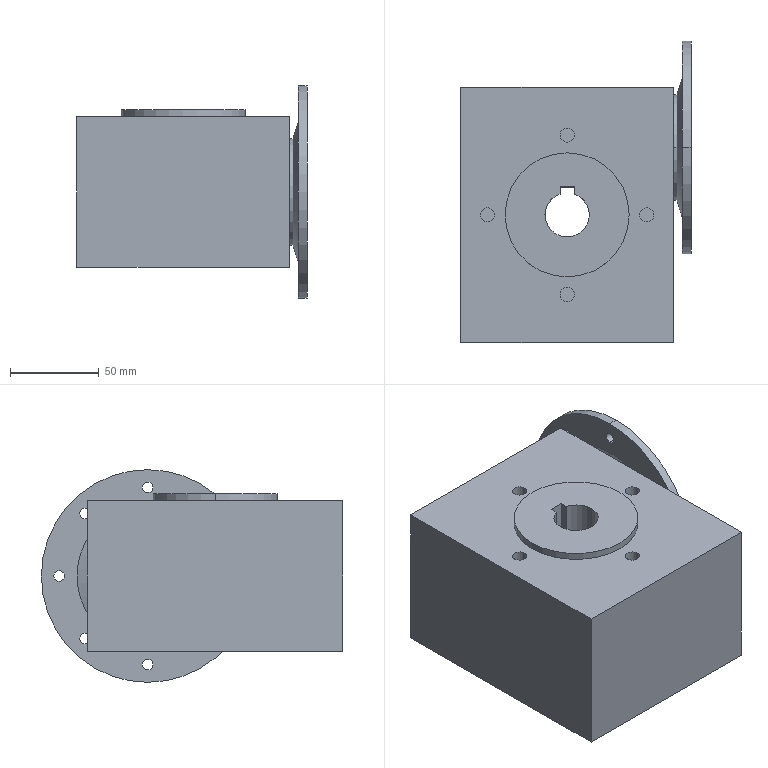Part | STEP file | Reducer | 1 solid | 51 faces | box 130 x 170 x 120 mm | volume 1507884 mm3 | cylinder 33 | plane 16 | cone 2 | commonest cylinder face diameters 6 x16 8 x8 25 x3 60 x2 70 x2 120 x2
STEP:
#1=CARTESIAN_POINT('',(12.5,0.,0.));
#2=VERTEX_POINT('',#1);
#3=CARTESIAN_POINT('',(-12.5,0.,0.));
#4=VERTEX_POINT('',#3);
#5=CARTESIAN_POINT('',(0.,0.,0.));
#6=DIRECTION('',(0.,0.,-1.));
#7=DIRECTION('',(1.,0.,0.));
#8=AXIS2_PLACEMENT_3D('',#5,#6,#7);
#9=CIRCLE('',#8,12.5);
#10=EDGE_CURVE('',#2,#4,#9,.T.);
#11=ORIENTED_EDGE('',*,*,#10,.T.);
#12=CARTESIAN_POINT('',(-12.5,0.,89.));
#13=VERTEX_POINT('',#12);
#14=CARTESIAN_POINT('',(-12.5,0.,-17.5));
#15=DIRECTION('',(0.,0.,1.));
#16=VECTOR('',#15,1000.);
#17=LINE('',#14,#16);
#18=EDGE_CURVE('',#4,#13,#17,.T.);
#19=ORIENTED_EDGE('',*,*,#18,.T.);
#20=CARTESIAN_POINT('',(12.5,0.,89.));
#21=VERTEX_POINT('',#20);
#22=CARTESIAN_POINT('',(0.,0.,89.));
#23=DIRECTION('',(0.,0.,-1.));
#24=DIRECTION('',(1.,0.,0.));
#25=AXIS2_PLACEMENT_3D('',#22,#23,#24);
#26=CIRCLE('',#25,12.5);
#27=EDGE_CURVE('',#21,#13,#26,.T.);
#28=ORIENTED_EDGE('',*,*,#27,.F.);
#29=CARTESIAN_POINT('',(12.5,0.,-17.5));
#30=DIRECTION('',(0.,0.,1.));
#31=VECTOR('',#30,1000.);
#32=LINE('',#29,#31);
#33=EDGE_CURVE('',#2,#21,#32,.T.);
#34=ORIENTED_EDGE('',*,*,#33,.F.);
#35=EDGE_LOOP('',(#11,#19,#28,#34));
#36=FACE_OUTER_BOUND('',#35,.T.);
#37=CARTESIAN_POINT('',(0.,0.,-17.5));
#38=DIRECTION('',(0.,0.,1.));
#39=DIRECTION('',(1.,0.,0.));
#40=AXIS2_PLACEMENT_3D('',#37,#38,#39);
#41=CYLINDRICAL_SURFACE('',#40,12.5);
#42=ADVANCED_FACE('',(#36),#41,.F.);
#43=CARTESIAN_POINT('',(4.,11.843,0.));
#44=VERTEX_POINT('',#43);
#45=CARTESIAN_POINT('',(0.,0.,0.));
#46=DIRECTION('',(0.,0.,-1.));
#47=DIRECTION('',(1.,0.,0.));
#48=AXIS2_PLACEMENT_3D('',#45,#46,#47);
#49=CIRCLE('',#48,12.5);
#50=EDGE_CURVE('',#44,#2,#49,.T.);
#51=ORIENTED_EDGE('',*,*,#50,.T.);
#52=ORIENTED_EDGE('',*,*,#33,.T.);
#53=CARTESIAN_POINT('',(4.,11.843,89.));
#54=VERTEX_POINT('',#53);
#55=CARTESIAN_POINT('',(0.,0.,89.));
#56=DIRECTION('',(0.,0.,-1.));
#57=DIRECTION('',(1.,0.,0.));
#58=AXIS2_PLACEMENT_3D('',#55,#56,#57);
#59=CIRCLE('',#58,12.5);
#60=EDGE_CURVE('',#54,#21,#59,.T.);
#61=ORIENTED_EDGE('',*,*,#60,.F.);
#62=CARTESIAN_POINT('',(4.,11.843,-17.5));
#63=DIRECTION('',(0.,0.,-1.));
#64=VECTOR('',#63,1000.);
#65=LINE('',#62,#64);
#66=EDGE_CURVE('',#54,#44,#65,.T.);
#67=ORIENTED_EDGE('',*,*,#66,.T.);
#68=EDGE_LOOP('',(#51,#52,#61,#67));
#69=FACE_OUTER_BOUND('',#68,.T.);
#70=CARTESIAN_POINT('',(0.,0.,-17.5));
#71=DIRECTION('',(0.,0.,1.));
#72=DIRECTION('',(1.,0.,0.));
#73=AXIS2_PLACEMENT_3D('',#70,#71,#72);
#74=CYLINDRICAL_SURFACE('',#73,12.5);
#75=ADVANCED_FACE('',(#69),#74,.F.);
#76=CARTESIAN_POINT('',(60.,38.,12.5));
#77=VERTEX_POINT('',#76);
#78=CARTESIAN_POINT('',(60.,38.,72.5));
#79=VERTEX_POINT('',#78);
#80=CARTESIAN_POINT('',(60.,38.,42.5));
#81=DIRECTION('',(1.,0.,0.));
#82=DIRECTION('',(0.,0.,-1.));
#83=AXIS2_PLACEMENT_3D('',#80,#81,#82);
#84=CIRCLE('',#83,30.);
#85=EDGE_CURVE('',#77,#79,#84,.T.);
#86=ORIENTED_EDGE('',*,*,#85,.T.);
#87=CARTESIAN_POINT('',(62.,38.,72.5));
#88=VERTEX_POINT('',#87);
#89=CARTESIAN_POINT('',(70.,38.,72.5));
#90=DIRECTION('',(1.,0.,0.));
#91=VECTOR('',#90,1000.);
#92=LINE('',#89,#91);
#93=EDGE_CURVE('',#79,#88,#92,.T.);
#94=ORIENTED_EDGE('',*,*,#93,.T.);
#95=CARTESIAN_POINT('',(62.,38.,12.5));
#96=VERTEX_POINT('',#95);
#97=CARTESIAN_POINT('',(62.,38.,42.5));
#98=DIRECTION('',(-1.,0.,0.));
#99=DIRECTION('',(0.,0.,-1.));
#100=AXIS2_PLACEMENT_3D('',#97,#98,#99);
#101=CIRCLE('',#100,30.);
#102=EDGE_CURVE('',#88,#96,#101,.T.);
#103=ORIENTED_EDGE('',*,*,#102,.T.);
#104=CARTESIAN_POINT('',(70.,38.,12.5));
#105=DIRECTION('',(1.,0.,0.));
#106=VECTOR('',#105,1000.);
#107=LINE('',#104,#106);
#108=EDGE_CURVE('',#77,#96,#107,.T.);
#109=ORIENTED_EDGE('',*,*,#108,.F.);
#110=EDGE_LOOP('',(#86,#94,#103,#109));
#111=FACE_OUTER_BOUND('',#110,.T.);
#112=CARTESIAN_POINT('',(70.,38.,42.5));
#113=DIRECTION('',(1.,0.,0.));
#114=DIRECTION('',(0.,0.,-1.));
#115=AXIS2_PLACEMENT_3D('',#112,#113,#114);
#116=CYLINDRICAL_SURFACE('',#115,30.);
#117=ADVANCED_FACE('',(#111),#116,.T.);
#118=CARTESIAN_POINT('',(35.,0.,89.));
#119=VERTEX_POINT('',#118);
#120=CARTESIAN_POINT('',(-35.,0.,89.));
#121=VERTEX_POINT('',#120);
#122=CARTESIAN_POINT('',(0.,0.,89.));
#123=DIRECTION('',(0.,0.,1.));
#124=DIRECTION('',(-1.,0.,0.));
#125=AXIS2_PLACEMENT_3D('',#122,#123,#124);
#126=CIRCLE('',#125,35.);
#127=EDGE_CURVE('',#119,#121,#126,.T.);
#128=ORIENTED_EDGE('',*,*,#127,.F.);
#129=CARTESIAN_POINT('',(35.,0.,85.));
#130=VERTEX_POINT('',#129);
#131=CARTESIAN_POINT('',(35.,0.,89.));
#132=DIRECTION('',(0.,0.,-1.));
#133=VECTOR('',#132,1000.);
#134=LINE('',#131,#133);
#135=EDGE_CURVE('',#119,#130,#134,.T.);
#136=ORIENTED_EDGE('',*,*,#135,.T.);
#137=CARTESIAN_POINT('',(-35.,0.,85.));
#138=VERTEX_POINT('',#137);
#139=CARTESIAN_POINT('',(0.,0.,85.));
#140=DIRECTION('',(0.,0.,-1.));
#141=DIRECTION('',(-1.,0.,0.));
#142=AXIS2_PLACEMENT_3D('',#139,#140,#141);
#143=CIRCLE('',#142,35.);
#144=EDGE_CURVE('',#138,#130,#143,.T.);
#145=ORIENTED_EDGE('',*,*,#144,.F.);
#146=CARTESIAN_POINT('',(-35.,0.,89.));
#147=DIRECTION('',(0.,0.,-1.));
#148=VECTOR('',#147,1000.);
#149=LINE('',#146,#148);
#150=EDGE_CURVE('',#121,#138,#149,.T.);
#151=ORIENTED_EDGE('',*,*,#150,.F.);
#152=EDGE_LOOP('',(#128,#136,#145,#151));
#153=FACE_OUTER_BOUND('',#152,.T.);
#154=CARTESIAN_POINT('',(0.,0.,89.));
#155=DIRECTION('',(0.,0.,-1.));
#156=DIRECTION('',(-1.,0.,0.));
#157=AXIS2_PLACEMENT_3D('',#154,#155,#156);
#158=CYLINDRICAL_SURFACE('',#157,35.);
#159=ADVANCED_FACE('',(#153),#158,.T.);
#160=CARTESIAN_POINT('',(-4.,45.,71.));
#161=VERTEX_POINT('',#160);
#162=CARTESIAN_POINT('',(4.,45.,71.));
#163=VERTEX_POINT('',#162);
#164=CARTESIAN_POINT('',(0.,45.,71.));
#165=DIRECTION('',(0.,0.,1.));
#166=DIRECTION('',(1.,0.,0.));
#167=AXIS2_PLACEMENT_3D('',#164,#165,#166);
#168=CIRCLE('',#167,4.);
#169=EDGE_CURVE('',#161,#163,#168,.T.);
#170=ORIENTED_EDGE('',*,*,#169,.F.);
#171=CARTESIAN_POINT('',(-4.,45.,85.));
#172=VERTEX_POINT('',#171);
#173=CARTESIAN_POINT('',(-4.,45.,71.));
#174=DIRECTION('',(0.,0.,1.));
#175=VECTOR('',#174,1000.);
#176=LINE('',#173,#175);
#177=EDGE_CURVE('',#161,#172,#176,.T.);
#178=ORIENTED_EDGE('',*,*,#177,.T.);
#179=CARTESIAN_POINT('',(4.,45.,85.));
#180=VERTEX_POINT('',#179);
#181=CARTESIAN_POINT('',(0.,45.,85.));
#182=DIRECTION('',(0.,0.,-1.));
#183=DIRECTION('',(1.,0.,0.));
#184=AXIS2_PLACEMENT_3D('',#181,#182,#183);
#185=CIRCLE('',#184,4.);
#186=EDGE_CURVE('',#180,#172,#185,.T.);
#187=ORIENTED_EDGE('',*,*,#186,.F.);
#188=CARTESIAN_POINT('',(4.,45.,71.));
#189=DIRECTION('',(0.,0.,1.));
#190=VECTOR('',#189,1000.);
#191=LINE('',#188,#190);
#192=EDGE_CURVE('',#163,#180,#191,.T.);
#193=ORIENTED_EDGE('',*,*,#192,.F.);
#194=EDGE_LOOP('',(#170,#178,#187,#193));
#195=FACE_OUTER_BOUND('',#194,.T.);
#196=CARTESIAN_POINT('',(0.,45.,71.));
#197=DIRECTION('',(0.,0.,1.));
#198=DIRECTION('',(1.,0.,0.));
#199=AXIS2_PLACEMENT_3D('',#196,#197,#198);
#200=CYLINDRICAL_SURFACE('',#199,4.);
#201=ADVANCED_FACE('',(#195),#200,.F.);
#202=CARTESIAN_POINT('',(-49.,0.,71.));
#203=VERTEX_POINT('',#202);
#204=CARTESIAN_POINT('',(-41.,0.,71.));
#205=VERTEX_POINT('',#204);
#206=CARTESIAN_POINT('',(-45.,0.,71.));
#207=DIRECTION('',(0.,0.,1.));
#208=DIRECTION('',(1.,0.,0.));
#209=AXIS2_PLACEMENT_3D('',#206,#207,#208);
#210=CIRCLE('',#209,4.);
#211=EDGE_CURVE('',#203,#205,#210,.T.);
#212=ORIENTED_EDGE('',*,*,#211,.F.);
#213=CARTESIAN_POINT('',(-49.,0.,85.));
#214=VERTEX_POINT('',#213);
#215=CARTESIAN_POINT('',(-49.,0.,71.));
#216=DIRECTION('',(0.,0.,1.));
#217=VECTOR('',#216,1000.);
#218=LINE('',#215,#217);
#219=EDGE_CURVE('',#203,#214,#218,.T.);
#220=ORIENTED_EDGE('',*,*,#219,.T.);
#221=CARTESIAN_POINT('',(-41.,0.,85.));
#222=VERTEX_POINT('',#221);
#223=CARTESIAN_POINT('',(-45.,0.,85.));
#224=DIRECTION('',(0.,0.,-1.));
#225=DIRECTION('',(1.,0.,0.));
#226=AXIS2_PLACEMENT_3D('',#223,#224,#225);
#227=CIRCLE('',#226,4.);
#228=EDGE_CURVE('',#222,#214,#227,.T.);
#229=ORIENTED_EDGE('',*,*,#228,.F.);
#230=CARTESIAN_POINT('',(-41.,0.,71.));
#231=DIRECTION('',(0.,0.,1.));
#232=VECTOR('',#231,1000.);
#233=LINE('',#230,#232);
#234=EDGE_CURVE('',#205,#222,#233,.T.);
#235=ORIENTED_EDGE('',*,*,#234,.F.);
#236=EDGE_LOOP('',(#212,#220,#229,#235));
#237=FACE_OUTER_BOUND('',#236,.T.);
#238=CARTESIAN_POINT('',(-45.,0.,71.));
#239=DIRECTION('',(0.,0.,1.));
#240=DIRECTION('',(1.,0.,0.));
#241=AXIS2_PLACEMENT_3D('',#238,#239,#240);
#242=CYLINDRICAL_SURFACE('',#241,4.);
#243=ADVANCED_FACE('',(#237),#242,.F.);
#244=CARTESIAN_POINT('',(41.,0.,71.));
#245=VERTEX_POINT('',#244);
#246=CARTESIAN_POINT('',(49.,0.,71.));
#247=VERTEX_POINT('',#246);
#248=CARTESIAN_POINT('',(45.,0.,71.));
#249=DIRECTION('',(0.,0.,1.));
#250=DIRECTION('',(1.,0.,0.));
#251=AXIS2_PLACEMENT_3D('',#248,#249,#250);
#252=CIRCLE('',#251,4.);
#253=EDGE_CURVE('',#245,#247,#252,.T.);
#254=ORIENTED_EDGE('',*,*,#253,.F.);
#255=CARTESIAN_POINT('',(41.,0.,85.));
#256=VERTEX_POINT('',#255);
#257=CARTESIAN_POINT('',(41.,0.,71.));
#258=DIRECTION('',(0.,0.,1.));
#259=VECTOR('',#258,1000.);
#260=LINE('',#257,#259);
#261=EDGE_CURVE('',#245,#256,#260,.T.);
#262=ORIENTED_EDGE('',*,*,#261,.T.);
#263=CARTESIAN_POINT('',(49.,0.,85.));
#264=VERTEX_POINT('',#263);
#265=CARTESIAN_POINT('',(45.,0.,85.));
#266=DIRECTION('',(0.,0.,-1.));
#267=DIRECTION('',(1.,0.,0.));
#268=AXIS2_PLACEMENT_3D('',#265,#266,#267);
#269=CIRCLE('',#268,4.);
#270=EDGE_CURVE('',#264,#256,#269,.T.);
#271=ORIENTED_EDGE('',*,*,#270,.F.);
#272=CARTESIAN_POINT('',(49.,0.,71.));
#273=DIRECTION('',(0.,0.,1.));
#274=VECTOR('',#273,1000.);
#275=LINE('',#272,#274);
#276=EDGE_CURVE('',#247,#264,#275,.T.);
#277=ORIENTED_EDGE('',*,*,#276,.F.);
#278=EDGE_LOOP('',(#254,#262,#271,#277));
#279=FACE_OUTER_BOUND('',#278,.T.);
#280=CARTESIAN_POINT('',(45.,0.,71.));
#281=DIRECTION('',(0.,0.,1.));
#282=DIRECTION('',(1.,0.,0.));
#283=AXIS2_PLACEMENT_3D('',#280,#281,#282);
#284=CYLINDRICAL_SURFACE('',#283,4.);
#285=ADVANCED_FACE('',(#279),#284,.F.);
#286=CARTESIAN_POINT('',(-4.,-45.,71.));
#287=VERTEX_POINT('',#286);
#288=CARTESIAN_POINT('',(4.,-45.,71.));
#289=VERTEX_POINT('',#288);
#290=CARTESIAN_POINT('',(0.,-45.,71.));
#291=DIRECTION('',(0.,0.,1.));
#292=DIRECTION('',(1.,0.,0.));
#293=AXIS2_PLACEMENT_3D('',#290,#291,#292);
#294=CIRCLE('',#293,4.);
#295=EDGE_CURVE('',#287,#289,#294,.T.);
#296=ORIENTED_EDGE('',*,*,#295,.F.);
#297=CARTESIAN_POINT('',(-4.,-45.,85.));
#298=VERTEX_POINT('',#297);
#299=CARTESIAN_POINT('',(-4.,-45.,71.));
#300=DIRECTION('',(0.,0.,1.));
#301=VECTOR('',#300,1000.);
#302=LINE('',#299,#301);
#303=EDGE_CURVE('',#287,#298,#302,.T.);
#304=ORIENTED_EDGE('',*,*,#303,.T.);
#305=CARTESIAN_POINT('',(4.,-45.,85.));
#306=VERTEX_POINT('',#305);
#307=CARTESIAN_POINT('',(0.,-45.,85.));
#308=DIRECTION('',(0.,0.,-1.));
#309=DIRECTION('',(1.,0.,0.));
#310=AXIS2_PLACEMENT_3D('',#307,#308,#309);
#311=CIRCLE('',#310,4.);
#312=EDGE_CURVE('',#306,#298,#311,.T.);
#313=ORIENTED_EDGE('',*,*,#312,.F.);
#314=CARTESIAN_POINT('',(4.,-45.,71.));
#315=DIRECTION('',(0.,0.,1.));
#316=VECTOR('',#315,1000.);
#317=LINE('',#314,#316);
#318=EDGE_CURVE('',#289,#306,#317,.T.);
#319=ORIENTED_EDGE('',*,*,#318,.F.);
#320=EDGE_LOOP('',(#296,#304,#313,#319));
#321=FACE_OUTER_BOUND('',#320,.T.);
#322=CARTESIAN_POINT('',(0.,-45.,71.));
#323=DIRECTION('',(0.,0.,1.));
#324=DIRECTION('',(1.,0.,0.));
#325=AXIS2_PLACEMENT_3D('',#322,#323,#324);
#326=CYLINDRICAL_SURFACE('',#325,4.);
#327=ADVANCED_FACE('',(#321),#326,.F.);
#328=ORIENTED_EDGE('',*,*,#102,.F.);
#329=CARTESIAN_POINT('',(65.,38.,82.5));
#330=VERTEX_POINT('',#329);
#331=CARTESIAN_POINT('',(65.,38.,82.5));
#332=DIRECTION('',(0.2873,0.,0.9578));
#333=VECTOR('',#332,1000.);
#334=LINE('',#331,#333);
#335=EDGE_CURVE('',#88,#330,#334,.T.);
#336=ORIENTED_EDGE('',*,*,#335,.T.);
#337=CARTESIAN_POINT('',(65.,38.,2.5));
#338=VERTEX_POINT('',#337);
#339=CARTESIAN_POINT('',(65.,38.,42.5));
#340=DIRECTION('',(-1.,0.,0.));
#341=DIRECTION('',(0.,0.,-1.));
#342=AXIS2_PLACEMENT_3D('',#339,#340,#341);
#343=CIRCLE('',#342,40.);
#344=EDGE_CURVE('',#330,#338,#343,.T.);
#345=ORIENTED_EDGE('',*,*,#344,.T.);
#346=CARTESIAN_POINT('',(65.,38.,2.5));
#347=DIRECTION('',(0.2873,0.,-0.9578));
#348=VECTOR('',#347,1000.);
#349=LINE('',#346,#348);
#350=EDGE_CURVE('',#96,#338,#349,.T.);
#351=ORIENTED_EDGE('',*,*,#350,.F.);
#352=EDGE_LOOP('',(#328,#336,#345,#351));
#353=FACE_OUTER_BOUND('',#352,.T.);
#354=CARTESIAN_POINT('',(65.,38.,42.5));
#355=DIRECTION('',(1.,0.,0.));
#356=DIRECTION('',(0.,0.,-1.));
#357=AXIS2_PLACEMENT_3D('',#354,#355,#356);
#358=CONICAL_SURFACE('',#357,40.,1.279);
#359=ADVANCED_FACE('',(#353),#358,.T.);
#360=CARTESIAN_POINT('',(65.,38.,102.5));
#361=VERTEX_POINT('',#360);
#362=CARTESIAN_POINT('',(65.,38.,-17.5));
#363=VERTEX_POINT('',#362);
#364=CARTESIAN_POINT('',(65.,38.,42.5));
#365=DIRECTION('',(-1.,0.,0.));
#366=DIRECTION('',(0.,0.,-1.));
#367=AXIS2_PLACEMENT_3D('',#364,#365,#366);
#368=CIRCLE('',#367,60.);
#369=EDGE_CURVE('',#361,#363,#368,.T.);
#370=ORIENTED_EDGE('',*,*,#369,.F.);
#371=CARTESIAN_POINT('',(70.,38.,102.5));
#372=VERTEX_POINT('',#371);
#373=CARTESIAN_POINT('',(70.,38.,102.5));
#374=DIRECTION('',(1.,0.,0.));
#375=VECTOR('',#374,1000.);
#376=LINE('',#373,#375);
#377=EDGE_CURVE('',#361,#372,#376,.T.);
#378=ORIENTED_EDGE('',*,*,#377,.T.);
#379=CARTESIAN_POINT('',(70.,38.,-17.5));
#380=VERTEX_POINT('',#379);
#381=CARTESIAN_POINT('',(70.,38.,42.5));
#382=DIRECTION('',(-1.,0.,0.));
#383=DIRECTION('',(0.,0.,-1.));
#384=AXIS2_PLACEMENT_3D('',#381,#382,#383);
#385=CIRCLE('',#384,60.);
#386=EDGE_CURVE('',#372,#380,#385,.T.);
#387=ORIENTED_EDGE('',*,*,#386,.T.);
#388=CARTESIAN_POINT('',(70.,38.,-17.5));
#389=DIRECTION('',(1.,0.,0.));
#390=VECTOR('',#389,1000.);
#391=LINE('',#388,#390);
#392=EDGE_CURVE('',#363,#380,#391,.T.);
#393=ORIENTED_EDGE('',*,*,#392,.F.);
#394=EDGE_LOOP('',(#370,#378,#387,#393));
#395=FACE_OUTER_BOUND('',#394,.T.);
#396=CARTESIAN_POINT('',(70.,38.,42.5));
#397=DIRECTION('',(1.,0.,0.));
#398=DIRECTION('',(0.,0.,-1.));
#399=AXIS2_PLACEMENT_3D('',#396,#397,#398);
#400=CYLINDRICAL_SURFACE('',#399,60.);
#401=ADVANCED_FACE('',(#395),#400,.T.);
#402=CARTESIAN_POINT('',(65.,88.,45.5));
#403=VERTEX_POINT('',#402);
#404=CARTESIAN_POINT('',(65.,88.,39.5));
#405=VERTEX_POINT('',#404);
#406=CARTESIAN_POINT('',(65.,88.,42.5));
#407=DIRECTION('',(1.,0.,0.));
#408=DIRECTION('',(0.,0.,-1.));
#409=AXIS2_PLACEMENT_3D('',#406,#407,#408);
#410=CIRCLE('',#409,3.);
#411=EDGE_CURVE('',#403,#405,#410,.T.);
#412=ORIENTED_EDGE('',*,*,#411,.F.);
#413=CARTESIAN_POINT('',(70.,88.,45.5));
#414=VERTEX_POINT('',#413);
#415=CARTESIAN_POINT('',(65.,88.,45.5));
#416=DIRECTION('',(1.,0.,0.));
#417=VECTOR('',#416,1000.);
#418=LINE('',#415,#417);
#419=EDGE_CURVE('',#403,#414,#418,.T.);
#420=ORIENTED_EDGE('',*,*,#419,.T.);
#421=CARTESIAN_POINT('',(70.,88.,39.5));
#422=VERTEX_POINT('',#421);
#423=CARTESIAN_POINT('',(70.,88.,42.5));
#424=DIRECTION('',(-1.,0.,0.));
#425=DIRECTION('',(0.,0.,-1.));
#426=AXIS2_PLACEMENT_3D('',#423,#424,#425);
#427=CIRCLE('',#426,3.);
#428=EDGE_CURVE('',#422,#414,#427,.T.);
#429=ORIENTED_EDGE('',*,*,#428,.F.);
#430=CARTESIAN_POINT('',(65.,88.,39.5));
#431=DIRECTION('',(1.,0.,0.));
#432=VECTOR('',#431,1000.);
#433=LINE('',#430,#432);
#434=EDGE_CURVE('',#405,#422,#433,.T.);
#435=ORIENTED_EDGE('',*,*,#434,.F.);
#436=EDGE_LOOP('',(#412,#420,#429,#435));
#437=FACE_OUTER_BOUND('',#436,.T.);
#438=CARTESIAN_POINT('',(65.,88.,42.5));
#439=DIRECTION('',(1.,0.,0.));
#440=DIRECTION('',(0.,0.,-1.));
#441=AXIS2_PLACEMENT_3D('',#438,#439,#440);
#442=CYLINDRICAL_SURFACE('',#441,3.);
#443=ADVANCED_FACE('',(#437),#442,.F.);
#444=CARTESIAN_POINT('',(65.,73.355,10.145));
#445=VERTEX_POINT('',#444);
#446=CARTESIAN_POINT('',(65.,73.355,4.145));
#447=VERTEX_POINT('',#446);
#448=CARTESIAN_POINT('',(65.,73.355,7.145));
#449=DIRECTION('',(1.,0.,0.));
#450=DIRECTION('',(0.,0.,-1.));
#451=AXIS2_PLACEMENT_3D('',#448,#449,#450);
#452=CIRCLE('',#451,3.);
#453=EDGE_CURVE('',#445,#447,#452,.T.);
#454=ORIENTED_EDGE('',*,*,#453,.F.);
#455=CARTESIAN_POINT('',(70.,73.355,10.145));
#456=VERTEX_POINT('',#455);
#457=CARTESIAN_POINT('',(65.,73.355,10.145));
#458=DIRECTION('',(1.,0.,0.));
#459=VECTOR('',#458,1000.);
#460=LINE('',#457,#459);
#461=EDGE_CURVE('',#445,#456,#460,.T.);
#462=ORIENTED_EDGE('',*,*,#461,.T.);
#463=CARTESIAN_POINT('',(70.,73.355,4.145));
#464=VERTEX_POINT('',#463);
#465=CARTESIAN_POINT('',(70.,73.355,7.145));
#466=DIRECTION('',(-1.,0.,0.));
#467=DIRECTION('',(0.,0.,-1.));
#468=AXIS2_PLACEMENT_3D('',#465,#466,#467);
#469=CIRCLE('',#468,3.);
#470=EDGE_CURVE('',#464,#456,#469,.T.);
#471=ORIENTED_EDGE('',*,*,#470,.F.);
#472=CARTESIAN_POINT('',(65.,73.355,4.145));
#473=DIRECTION('',(1.,0.,0.));
#474=VECTOR('',#473,1000.);
#475=LINE('',#472,#474);
#476=EDGE_CURVE('',#447,#464,#475,.T.);
#477=ORIENTED_EDGE('',*,*,#476,.F.);
#478=EDGE_LOOP('',(#454,#462,#471,#477));
#479=FACE_OUTER_BOUND('',#478,.T.);
#480=CARTESIAN_POINT('',(65.,73.355,7.145));
#481=DIRECTION('',(1.,0.,0.));
#482=DIRECTION('',(0.,0.,-1.));
#483=AXIS2_PLACEMENT_3D('',#480,#481,#482);
#484=CYLINDRICAL_SURFACE('',#483,3.);
#485=ADVANCED_FACE('',(#479),#484,.F.);
#486=CARTESIAN_POINT('',(65.,38.,-4.5));
#487=VERTEX_POINT('',#486);
#488=CARTESIAN_POINT('',(65.,38.,-10.5));
#489=VERTEX_POINT('',#488);
#490=CARTESIAN_POINT('',(65.,38.,-7.5));
#491=DIRECTION('',(1.,0.,0.));
#492=DIRECTION('',(0.,0.,-1.));
#493=AXIS2_PLACEMENT_3D('',#490,#491,#492);
#494=CIRCLE('',#493,3.);
#495=EDGE_CURVE('',#487,#489,#494,.T.);
#496=ORIENTED_EDGE('',*,*,#495,.F.);
#497=CARTESIAN_POINT('',(70.,38.,-4.5));
#498=VERTEX_POINT('',#497);
#499=CARTESIAN_POINT('',(65.,38.,-4.5));
#500=DIRECTION('',(1.,0.,0.));
#501=VECTOR('',#500,1000.);
#502=LINE('',#499,#501);
#503=EDGE_CURVE('',#487,#498,#502,.T.);
#504=ORIENTED_EDGE('',*,*,#503,.T.);
#505=CARTESIAN_POINT('',(70.,38.,-10.5));
#506=VERTEX_POINT('',#505);
#507=CARTESIAN_POINT('',(70.,38.,-7.5));
#508=DIRECTION('',(-1.,0.,0.));
#509=DIRECTION('',(0.,0.,-1.));
#510=AXIS2_PLACEMENT_3D('',#507,#508,#509);
#511=CIRCLE('',#510,3.);
#512=EDGE_CURVE('',#506,#498,#511,.T.);
#513=ORIENTED_EDGE('',*,*,#512,.F.);
#514=CARTESIAN_POINT('',(65.,38.,-10.5));
#515=DIRECTION('',(1.,0.,0.));
#516=VECTOR('',#515,1000.);
#517=LINE('',#514,#516);
#518=EDGE_CURVE('',#489,#506,#517,.T.);
#519=ORIENTED_EDGE('',*,*,#518,.F.);
#520=EDGE_LOOP('',(#496,#504,#513,#519));
#521=FACE_OUTER_BOUND('',#520,.T.);
#522=CARTESIAN_POINT('',(65.,38.,-7.5));
#523=DIRECTION('',(1.,0.,0.));
#524=DIRECTION('',(0.,0.,-1.));
#525=AXIS2_PLACEMENT_3D('',#522,#523,#524);
#526=CYLINDRICAL_SURFACE('',#525,3.);
#527=ADVANCED_FACE('',(#521),#526,.F.);
#528=CARTESIAN_POINT('',(65.,2.645,10.145));
#529=VERTEX_POINT('',#528);
#530=CARTESIAN_POINT('',(65.,2.645,4.145));
#531=VERTEX_POINT('',#530);
#532=CARTESIAN_POINT('',(65.,2.645,7.145));
#533=DIRECTION('',(1.,0.,0.));
#534=DIRECTION('',(0.,0.,-1.));
#535=AXIS2_PLACEMENT_3D('',#532,#533,#534);
#536=CIRCLE('',#535,3.);
#537=EDGE_CURVE('',#529,#531,#536,.T.);
#538=ORIENTED_EDGE('',*,*,#537,.F.);
#539=CARTESIAN_POINT('',(70.,2.645,10.145));
#540=VERTEX_POINT('',#539);
#541=CARTESIAN_POINT('',(65.,2.645,10.145));
#542=DIRECTION('',(1.,0.,0.));
#543=VECTOR('',#542,1000.);
#544=LINE('',#541,#543);
#545=EDGE_CURVE('',#529,#540,#544,.T.);
#546=ORIENTED_EDGE('',*,*,#545,.T.);
#547=CARTESIAN_POINT('',(70.,2.645,4.145));
#548=VERTEX_POINT('',#547);
#549=CARTESIAN_POINT('',(70.,2.645,7.145));
#550=DIRECTION('',(-1.,0.,0.));
#551=DIRECTION('',(0.,0.,-1.));
#552=AXIS2_PLACEMENT_3D('',#549,#550,#551);
#553=CIRCLE('',#552,3.);
#554=EDGE_CURVE('',#548,#540,#553,.T.);
#555=ORIENTED_EDGE('',*,*,#554,.F.);
#556=CARTESIAN_POINT('',(65.,2.645,4.145));
#557=DIRECTION('',(1.,0.,0.));
#558=VECTOR('',#557,1000.);
#559=LINE('',#556,#558);
#560=EDGE_CURVE('',#531,#548,#559,.T.);
#561=ORIENTED_EDGE('',*,*,#560,.F.);
#562=EDGE_LOOP('',(#538,#546,#555,#561));
#563=FACE_OUTER_BOUND('',#562,.T.);
#564=CARTESIAN_POINT('',(65.,2.645,7.145));
#565=DIRECTION('',(1.,0.,0.));
#566=DIRECTION('',(0.,0.,-1.));
#567=AXIS2_PLACEMENT_3D('',#564,#565,#566);
#568=CYLINDRICAL_SURFACE('',#567,3.);
#569=ADVANCED_FACE('',(#563),#568,.F.);
#570=CARTESIAN_POINT('',(65.,-12.,45.5));
#571=VERTEX_POINT('',#570);
#572=CARTESIAN_POINT('',(65.,-12.,39.5));
#573=VERTEX_POINT('',#572);
#574=CARTESIAN_POINT('',(65.,-12.,42.5));
#575=DIRECTION('',(1.,0.,0.));
#576=DIRECTION('',(0.,0.,-1.));
#577=AXIS2_PLACEMENT_3D('',#574,#575,#576);
#578=CIRCLE('',#577,3.);
#579=EDGE_CURVE('',#571,#573,#578,.T.);
#580=ORIENTED_EDGE('',*,*,#579,.F.);
#581=CARTESIAN_POINT('',(70.,-12.,45.5));
#582=VERTEX_POINT('',#581);
#583=CARTESIAN_POINT('',(65.,-12.,45.5));
#584=DIRECTION('',(1.,0.,0.));
#585=VECTOR('',#584,1000.);
#586=LINE('',#583,#585);
#587=EDGE_CURVE('',#571,#582,#586,.T.);
#588=ORIENTED_EDGE('',*,*,#587,.T.);
#589=CARTESIAN_POINT('',(70.,-12.,39.5));
#590=VERTEX_POINT('',#589);
#591=CARTESIAN_POINT('',(70.,-12.,42.5));
#592=DIRECTION('',(-1.,0.,0.));
#593=DIRECTION('',(0.,0.,-1.));
#594=AXIS2_PLACEMENT_3D('',#591,#592,#593);
#595=CIRCLE('',#594,3.);
#596=EDGE_CURVE('',#590,#582,#595,.T.);
#597=ORIENTED_EDGE('',*,*,#596,.F.);
#598=CARTESIAN_POINT('',(65.,-12.,39.5));
#599=DIRECTION('',(1.,0.,0.));
#600=VECTOR('',#599,1000.);
#601=LINE('',#598,#600);
#602=EDGE_CURVE('',#573,#590,#601,.T.);
#603=ORIENTED_EDGE('',*,*,#602,.F.);
#604=EDGE_LOOP('',(#580,#588,#597,#603));
#605=FACE_OUTER_BOUND('',#604,.T.);
#606=CARTESIAN_POINT('',(65.,-12.,42.5));
#607=DIRECTION('',(1.,0.,0.));
#608=DIRECTION('',(0.,0.,-1.));
#609=AXIS2_PLACEMENT_3D('',#606,#607,#608);
#610=CYLINDRICAL_SURFACE('',#609,3.);
#611=ADVANCED_FACE('',(#605),#610,.F.);
#612=CARTESIAN_POINT('',(65.,2.645,80.855));
#613=VERTEX_POINT('',#612);
#614=CARTESIAN_POINT('',(65.,2.645,74.855));
#615=VERTEX_POINT('',#614);
#616=CARTESIAN_POINT('',(65.,2.645,77.855));
#617=DIRECTION('',(1.,0.,0.));
#618=DIRECTION('',(0.,0.,-1.));
#619=AXIS2_PLACEMENT_3D('',#616,#617,#618);
#620=CIRCLE('',#619,3.);
#621=EDGE_CURVE('',#613,#615,#620,.T.);
#622=ORIENTED_EDGE('',*,*,#621,.F.);
#623=CARTESIAN_POINT('',(70.,2.645,80.855));
#624=VERTEX_POINT('',#623);
#625=CARTESIAN_POINT('',(65.,2.645,80.855));
#626=DIRECTION('',(1.,0.,0.));
#627=VECTOR('',#626,1000.);
#628=LINE('',#625,#627);
#629=EDGE_CURVE('',#613,#624,#628,.T.);
#630=ORIENTED_EDGE('',*,*,#629,.T.);
#631=CARTESIAN_POINT('',(70.,2.645,74.855));
#632=VERTEX_POINT('',#631);
#633=CARTESIAN_POINT('',(70.,2.645,77.855));
#634=DIRECTION('',(-1.,0.,0.));
#635=DIRECTION('',(0.,0.,-1.));
#636=AXIS2_PLACEMENT_3D('',#633,#634,#635);
#637=CIRCLE('',#636,3.);
#638=EDGE_CURVE('',#632,#624,#637,.T.);
#639=ORIENTED_EDGE('',*,*,#638,.F.);
#640=CARTESIAN_POINT('',(65.,2.645,74.855));
#641=DIRECTION('',(1.,0.,0.));
#642=VECTOR('',#641,1000.);
#643=LINE('',#640,#642);
#644=EDGE_CURVE('',#615,#632,#643,.T.);
#645=ORIENTED_EDGE('',*,*,#644,.F.);
#646=EDGE_LOOP('',(#622,#630,#639,#645));
#647=FACE_OUTER_BOUND('',#646,.T.);
#648=CARTESIAN_POINT('',(65.,2.645,77.855));
#649=DIRECTION('',(1.,0.,0.));
#650=DIRECTION('',(0.,0.,-1.));
#651=AXIS2_PLACEMENT_3D('',#648,#649,#650);
#652=CYLINDRICAL_SURFACE('',#651,3.);
#653=ADVANCED_FACE('',(#647),#652,.F.);
#654=CARTESIAN_POINT('',(65.,38.,95.5));
#655=VERTEX_POINT('',#654);
#656=CARTESIAN_POINT('',(65.,38.,89.5));
#657=VERTEX_POINT('',#656);
#658=CARTESIAN_POINT('',(65.,38.,92.5));
#659=DIRECTION('',(1.,0.,0.));
#660=DIRECTION('',(0.,0.,-1.));
#661=AXIS2_PLACEMENT_3D('',#658,#659,#660);
#662=CIRCLE('',#661,3.);
#663=EDGE_CURVE('',#655,#657,#662,.T.);
#664=ORIENTED_EDGE('',*,*,#663,.F.);
#665=CARTESIAN_POINT('',(70.,38.,95.5));
#666=VERTEX_POINT('',#665);
#667=CARTESIAN_POINT('',(65.,38.,95.5));
#668=DIRECTION('',(1.,0.,0.));
#669=VECTOR('',#668,1000.);
#670=LINE('',#667,#669);
#671=EDGE_CURVE('',#655,#666,#670,.T.);
#672=ORIENTED_EDGE('',*,*,#671,.T.);
#673=CARTESIAN_POINT('',(70.,38.,89.5));
#674=VERTEX_POINT('',#673);
#675=CARTESIAN_POINT('',(70.,38.,92.5));
#676=DIRECTION('',(-1.,0.,0.));
#677=DIRECTION('',(0.,0.,-1.));
#678=AXIS2_PLACEMENT_3D('',#675,#676,#677);
#679=CIRCLE('',#678,3.);
#680=EDGE_CURVE('',#674,#666,#679,.T.);
#681=ORIENTED_EDGE('',*,*,#680,.F.);
#682=CARTESIAN_POINT('',(65.,38.,89.5));
#683=DIRECTION('',(1.,0.,0.));
#684=VECTOR('',#683,1000.);
#685=LINE('',#682,#684);
#686=EDGE_CURVE('',#657,#674,#685,.T.);
#687=ORIENTED_EDGE('',*,*,#686,.F.);
#688=EDGE_LOOP('',(#664,#672,#681,#687));
#689=FACE_OUTER_BOUND('',#688,.T.);
#690=CARTESIAN_POINT('',(65.,38.,92.5));
#691=DIRECTION('',(1.,0.,0.));
#692=DIRECTION('',(0.,0.,-1.));
#693=AXIS2_PLACEMENT_3D('',#690,#691,#692);
#694=CYLINDRICAL_SURFACE('',#693,3.);
#695=ADVANCED_FACE('',(#689),#694,.F.);
#696=CARTESIAN_POINT('',(65.,73.355,80.855));
#697=VERTEX_POINT('',#696);
#698=CARTESIAN_POINT('',(65.,73.355,74.855));
#699=VERTEX_POINT('',#698);
#700=CARTESIAN_POINT('',(65.,73.355,77.855));
#701=DIRECTION('',(1.,0.,0.));
#702=DIRECTION('',(0.,0.,-1.));
#703=AXIS2_PLACEMENT_3D('',#700,#701,#702);
#704=CIRCLE('',#703,3.);
#705=EDGE_CURVE('',#697,#699,#704,.T.);
#706=ORIENTED_EDGE('',*,*,#705,.F.);
#707=CARTESIAN_POINT('',(70.,73.355,80.855));
#708=VERTEX_POINT('',#707);
#709=CARTESIAN_POINT('',(65.,73.355,80.855));
#710=DIRECTION('',(1.,0.,0.));
#711=VECTOR('',#710,1000.);
#712=LINE('',#709,#711);
#713=EDGE_CURVE('',#697,#708,#712,.T.);
#714=ORIENTED_EDGE('',*,*,#713,.T.);
#715=CARTESIAN_POINT('',(70.,73.355,74.855));
#716=VERTEX_POINT('',#715);
#717=CARTESIAN_POINT('',(70.,73.355,77.855));
#718=DIRECTION('',(-1.,0.,0.));
#719=DIRECTION('',(0.,0.,-1.));
#720=AXIS2_PLACEMENT_3D('',#717,#718,#719);
#721=CIRCLE('',#720,3.);
#722=EDGE_CURVE('',#716,#708,#721,.T.);
#723=ORIENTED_EDGE('',*,*,#722,.F.);
#724=CARTESIAN_POINT('',(65.,73.355,74.855));
#725=DIRECTION('',(1.,0.,0.));
#726=VECTOR('',#725,1000.);
#727=LINE('',#724,#726);
#728=EDGE_CURVE('',#699,#716,#727,.T.);
#729=ORIENTED_EDGE('',*,*,#728,.F.);
#730=EDGE_LOOP('',(#706,#714,#723,#729));
#731=FACE_OUTER_BOUND('',#730,.T.);
#732=CARTESIAN_POINT('',(65.,73.355,77.855));
#733=DIRECTION('',(1.,0.,0.));
#734=DIRECTION('',(0.,0.,-1.));
#735=AXIS2_PLACEMENT_3D('',#732,#733,#734);
#736=CYLINDRICAL_SURFACE('',#735,3.);
#737=ADVANCED_FACE('',(#731),#736,.F.);
#738=CARTESIAN_POINT('',(60.,72.,0.));
#739=VERTEX_POINT('',#738);
#740=CARTESIAN_POINT('',(-60.,72.,0.));
#741=VERTEX_POINT('',#740);
#742=CARTESIAN_POINT('',(-60.,72.,0.));
#743=DIRECTION('',(-1.,0.,0.));
#744=VECTOR('',#743,1000.);
#745=LINE('',#742,#744);
#746=EDGE_CURVE('',#739,#741,#745,.T.);
#747=ORIENTED_EDGE('',*,*,#746,.F.);
#748=CARTESIAN_POINT('',(60.,-72.,0.));
#749=VERTEX_POINT('',#748);
#750=CARTESIAN_POINT('',(60.,-72.,0.));
#751=DIRECTION('',(0.,1.,0.));
#752=VECTOR('',#751,1000.);
#753=LINE('',#750,#752);
#754=EDGE_CURVE('',#749,#739,#753,.T.);
#755=ORIENTED_EDGE('',*,*,#754,.F.);
#756=CARTESIAN_POINT('',(-60.,-72.,0.));
#757=VERTEX_POINT('',#756);
#758=CARTESIAN_POINT('',(-60.,-72.,0.));
#759=DIRECTION('',(1.,0.,0.));
#760=VECTOR('',#759,1000.);
#761=LINE('',#758,#760);
#762=EDGE_CURVE('',#757,#749,#761,.T.);
#763=ORIENTED_EDGE('',*,*,#762,.F.);
#764=CARTESIAN_POINT('',(-60.,-72.,0.));
#765=DIRECTION('',(0.,-1.,0.));
#766=VECTOR('',#765,1000.);
#767=LINE('',#764,#766);
#768=EDGE_CURVE('',#741,#757,#767,.T.);
#769=ORIENTED_EDGE('',*,*,#768,.F.);
#770=EDGE_LOOP('',(#747,#755,#763,#769));
#771=FACE_OUTER_BOUND('',#770,.T.);
#772=CARTESIAN_POINT('',(-4.,15.8,0.));
#773=VERTEX_POINT('',#772);
#774=CARTESIAN_POINT('',(4.,15.8,0.));
#775=VERTEX_POINT('',#774);
#776=CARTESIAN_POINT('',(-60.,15.8,0.));
#777=DIRECTION('',(1.,0.,0.));
#778=VECTOR('',#777,1000.);
#779=LINE('',#776,#778);
#780=EDGE_CURVE('',#773,#775,#779,.T.);
#781=ORIENTED_EDGE('',*,*,#780,.F.);
#782=CARTESIAN_POINT('',(-4.,11.843,0.));
#783=VERTEX_POINT('',#782);
#784=CARTESIAN_POINT('',(-4.,-72.,0.));
#785=DIRECTION('',(0.,1.,0.));
#786=VECTOR('',#785,1000.);
#787=LINE('',#784,#786);
#788=EDGE_CURVE('',#783,#773,#787,.T.);
#789=ORIENTED_EDGE('',*,*,#788,.F.);
#790=CARTESIAN_POINT('',(0.,0.,0.));
#791=DIRECTION('',(0.,0.,-1.));
#792=DIRECTION('',(1.,0.,0.));
#793=AXIS2_PLACEMENT_3D('',#790,#791,#792);
#794=CIRCLE('',#793,12.5);
#795=EDGE_CURVE('',#4,#783,#794,.T.);
#796=ORIENTED_EDGE('',*,*,#795,.F.);
#797=ORIENTED_EDGE('',*,*,#10,.F.);
#798=ORIENTED_EDGE('',*,*,#50,.F.);
#799=CARTESIAN_POINT('',(4.,-72.,0.));
#800=DIRECTION('',(0.,-1.,0.));
#801=VECTOR('',#800,1000.);
#802=LINE('',#799,#801);
#803=EDGE_CURVE('',#775,#44,#802,.T.);
#804=ORIENTED_EDGE('',*,*,#803,.F.);
#805=EDGE_LOOP('',(#781,#789,#796,#797,#798,#804));
#806=FACE_BOUND('',#805,.T.);
#807=CARTESIAN_POINT('',(-60.,-72.,0.));
#808=DIRECTION('',(0.,0.,1.));
#809=DIRECTION('',(1.,0.,0.));
#810=AXIS2_PLACEMENT_3D('',#807,#808,#809);
#811=PLANE('',#810);
#812=ADVANCED_FACE('',(#771,#806),#811,.F.);
#813=CARTESIAN_POINT('',(-60.,-72.,85.));
#814=VERTEX_POINT('',#813);
#815=CARTESIAN_POINT('',(-60.,-72.,85.));
#816=DIRECTION('',(0.,0.,-1.));
#817=VECTOR('',#816,1000.);
#818=LINE('',#815,#817);
#819=EDGE_CURVE('',#814,#757,#818,.T.);
#820=ORIENTED_EDGE('',*,*,#819,.F.);
#821=CARTESIAN_POINT('',(-60.,72.,85.));
#822=VERTEX_POINT('',#821);
#823=CARTESIAN_POINT('',(-60.,72.,85.));
#824=DIRECTION('',(0.,-1.,0.));
#825=VECTOR('',#824,1000.);
#826=LINE('',#823,#825);
#827=EDGE_CURVE('',#822,#814,#826,.T.);
#828=ORIENTED_EDGE('',*,*,#827,.F.);
#829=CARTESIAN_POINT('',(-60.,72.,85.));
#830=DIRECTION('',(0.,0.,1.));
#831=VECTOR('',#830,1000.);
#832=LINE('',#829,#831);
#833=EDGE_CURVE('',#741,#822,#832,.T.);
#834=ORIENTED_EDGE('',*,*,#833,.F.);
#835=ORIENTED_EDGE('',*,*,#768,.T.);
#836=EDGE_LOOP('',(#820,#828,#834,#835));
#837=FACE_OUTER_BOUND('',#836,.T.);
#838=CARTESIAN_POINT('',(-60.,72.,85.));
#839=DIRECTION('',(1.,0.,0.));
#840=DIRECTION('',(0.,0.,-1.));
#841=AXIS2_PLACEMENT_3D('',#838,#839,#840);
#842=PLANE('',#841);
#843=ADVANCED_FACE('',(#837),#842,.F.);
#844=ORIENTED_EDGE('',*,*,#833,.T.);
#845=CARTESIAN_POINT('',(60.,72.,85.));
#846=VERTEX_POINT('',#845);
#847=CARTESIAN_POINT('',(-60.,72.,85.));
#848=DIRECTION('',(-1.,0.,0.));
#849=VECTOR('',#848,1000.);
#850=LINE('',#847,#849);
#851=EDGE_CURVE('',#846,#822,#850,.T.);
#852=ORIENTED_EDGE('',*,*,#851,.F.);
#853=CARTESIAN_POINT('',(60.,72.,85.));
#854=DIRECTION('',(0.,0.,1.));
#855=VECTOR('',#854,1000.);
#856=LINE('',#853,#855);
#857=EDGE_CURVE('',#739,#846,#856,.T.);
#858=ORIENTED_EDGE('',*,*,#857,.F.);
#859=ORIENTED_EDGE('',*,*,#746,.T.);
#860=EDGE_LOOP('',(#844,#852,#858,#859));
#861=FACE_OUTER_BOUND('',#860,.T.);
#862=CARTESIAN_POINT('',(-60.,72.,85.));
#863=DIRECTION('',(0.,-1.,0.));
#864=DIRECTION('',(0.,0.,-1.));
#865=AXIS2_PLACEMENT_3D('',#862,#863,#864);
#866=PLANE('',#865);
#867=ADVANCED_FACE('',(#861),#866,.F.);
#868=ORIENTED_EDGE('',*,*,#857,.T.);
#869=CARTESIAN_POINT('',(60.,-72.,85.));
#870=VERTEX_POINT('',#869);
#871=CARTESIAN_POINT('',(60.,72.,85.));
#872=DIRECTION('',(0.,1.,0.));
#873=VECTOR('',#872,1000.);
#874=LINE('',#871,#873);
#875=EDGE_CURVE('',#870,#846,#874,.T.);
#876=ORIENTED_EDGE('',*,*,#875,.F.);
#877=CARTESIAN_POINT('',(60.,-72.,85.));
#878=DIRECTION('',(0.,0.,1.));
#879=VECTOR('',#878,1000.);
#880=LINE('',#877,#879);
#881=EDGE_CURVE('',#749,#870,#880,.T.);
#882=ORIENTED_EDGE('',*,*,#881,.F.);
#883=ORIENTED_EDGE('',*,*,#754,.T.);
#884=EDGE_LOOP('',(#868,#876,#882,#883));
#885=FACE_OUTER_BOUND('',#884,.T.);
#886=ORIENTED_EDGE('',*,*,#85,.F.);
#887=CARTESIAN_POINT('',(60.,38.,42.5));
#888=DIRECTION('',(1.,0.,0.));
#889=DIRECTION('',(0.,0.,-1.));
#890=AXIS2_PLACEMENT_3D('',#887,#888,#889);
#891=CIRCLE('',#890,30.);
#892=EDGE_CURVE('',#79,#77,#891,.T.);
#893=ORIENTED_EDGE('',*,*,#892,.F.);
#894=EDGE_LOOP('',(#886,#893));
#895=FACE_BOUND('',#894,.T.);
#896=CARTESIAN_POINT('',(60.,72.,85.));
#897=DIRECTION('',(-1.,0.,0.));
#898=DIRECTION('',(0.,0.,1.));
#899=AXIS2_PLACEMENT_3D('',#896,#897,#898);
#900=PLANE('',#899);
#901=ADVANCED_FACE('',(#885,#895),#900,.F.);
#902=ORIENTED_EDGE('',*,*,#881,.T.);
#903=CARTESIAN_POINT('',(-60.,-72.,85.));
#904=DIRECTION('',(1.,0.,0.));
#905=VECTOR('',#904,1000.);
#906=LINE('',#903,#905);
#907=EDGE_CURVE('',#814,#870,#906,.T.);
#908=ORIENTED_EDGE('',*,*,#907,.F.);
#909=ORIENTED_EDGE('',*,*,#819,.T.);
#910=ORIENTED_EDGE('',*,*,#762,.T.);
#911=EDGE_LOOP('',(#902,#908,#909,#910));
#912=FACE_OUTER_BOUND('',#911,.T.);
#913=CARTESIAN_POINT('',(-60.,-72.,85.));
#914=DIRECTION('',(0.,1.,0.));
#915=DIRECTION('',(0.,0.,1.));
#916=AXIS2_PLACEMENT_3D('',#913,#914,#915);
#917=PLANE('',#916);
#918=ADVANCED_FACE('',(#912),#917,.F.);
#919=CARTESIAN_POINT('',(4.,15.8,89.));
#920=VERTEX_POINT('',#919);
#921=CARTESIAN_POINT('',(4.,15.8,89.));
#922=DIRECTION('',(0.,-1.,0.));
#923=VECTOR('',#922,1000.);
#924=LINE('',#921,#923);
#925=EDGE_CURVE('',#920,#54,#924,.T.);
#926=ORIENTED_EDGE('',*,*,#925,.F.);
#927=CARTESIAN_POINT('',(4.,15.8,-17.5));
#928=DIRECTION('',(0.,0.,1.));
#929=VECTOR('',#928,1000.);
#930=LINE('',#927,#929);
#931=EDGE_CURVE('',#775,#920,#930,.T.);
#932=ORIENTED_EDGE('',*,*,#931,.F.);
#933=ORIENTED_EDGE('',*,*,#803,.T.);
#934=ORIENTED_EDGE('',*,*,#66,.F.);
#935=EDGE_LOOP('',(#926,#932,#933,#934));
#936=FACE_OUTER_BOUND('',#935,.T.);
#937=CARTESIAN_POINT('',(4.,15.8,-17.5));
#938=DIRECTION('',(1.,0.,0.));
#939=DIRECTION('',(0.,0.,-1.));
#940=AXIS2_PLACEMENT_3D('',#937,#938,#939);
#941=PLANE('',#940);
#942=ADVANCED_FACE('',(#936),#941,.F.);
#943=CARTESIAN_POINT('',(-4.,15.8,89.));
#944=VERTEX_POINT('',#943);
#945=CARTESIAN_POINT('',(-4.,15.8,89.));
#946=DIRECTION('',(1.,0.,0.));
#947=VECTOR('',#946,1000.);
#948=LINE('',#945,#947);
#949=EDGE_CURVE('',#944,#920,#948,.T.);
#950=ORIENTED_EDGE('',*,*,#949,.F.);
#951=CARTESIAN_POINT('',(-4.,15.8,-17.5));
#952=DIRECTION('',(0.,0.,1.));
#953=VECTOR('',#952,1000.);
#954=LINE('',#951,#953);
#955=EDGE_CURVE('',#773,#944,#954,.T.);
#956=ORIENTED_EDGE('',*,*,#955,.F.);
#957=ORIENTED_EDGE('',*,*,#780,.T.);
#958=ORIENTED_EDGE('',*,*,#931,.T.);
#959=EDGE_LOOP('',(#950,#956,#957,#958));
#960=FACE_OUTER_BOUND('',#959,.T.);
#961=CARTESIAN_POINT('',(-4.,15.8,-17.5));
#962=DIRECTION('',(0.,1.,0.));
#963=DIRECTION('',(0.,0.,1.));
#964=AXIS2_PLACEMENT_3D('',#961,#962,#963);
#965=PLANE('',#964);
#966=ADVANCED_FACE('',(#960),#965,.F.);
#967=CARTESIAN_POINT('',(-4.,11.843,89.));
#968=VERTEX_POINT('',#967);
#969=CARTESIAN_POINT('',(-4.,11.843,89.));
#970=DIRECTION('',(0.,1.,0.));
#971=VECTOR('',#970,1000.);
#972=LINE('',#969,#971);
#973=EDGE_CURVE('',#968,#944,#972,.T.);
#974=ORIENTED_EDGE('',*,*,#973,.F.);
#975=CARTESIAN_POINT('',(-4.,11.843,-17.5));
#976=DIRECTION('',(0.,0.,1.));
#977=VECTOR('',#976,1000.);
#978=LINE('',#975,#977);
#979=EDGE_CURVE('',#783,#968,#978,.T.);
#980=ORIENTED_EDGE('',*,*,#979,.F.);
#981=ORIENTED_EDGE('',*,*,#788,.T.);
#982=ORIENTED_EDGE('',*,*,#955,.T.);
#983=EDGE_LOOP('',(#974,#980,#981,#982));
#984=FACE_OUTER_BOUND('',#983,.T.);
#985=CARTESIAN_POINT('',(-4.,11.843,-17.5));
#986=DIRECTION('',(-1.,0.,0.));
#987=DIRECTION('',(0.,0.,1.));
#988=AXIS2_PLACEMENT_3D('',#985,#986,#987);
#989=PLANE('',#988);
#990=ADVANCED_FACE('',(#984),#989,.F.);
#991=ORIENTED_EDGE('',*,*,#18,.F.);
#992=ORIENTED_EDGE('',*,*,#795,.T.);
#993=ORIENTED_EDGE('',*,*,#979,.T.);
#994=CARTESIAN_POINT('',(0.,0.,89.));
#995=DIRECTION('',(0.,0.,-1.));
#996=DIRECTION('',(1.,0.,0.));
#997=AXIS2_PLACEMENT_3D('',#994,#995,#996);
#998=CIRCLE('',#997,12.5);
#999=EDGE_CURVE('',#13,#968,#998,.T.);
#1000=ORIENTED_EDGE('',*,*,#999,.F.);
#1001=EDGE_LOOP('',(#991,#992,#993,#1000));
#1002=FACE_OUTER_BOUND('',#1001,.T.);
#1003=CARTESIAN_POINT('',(0.,0.,-17.5));
#1004=DIRECTION('',(0.,0.,1.));
#1005=DIRECTION('',(1.,0.,0.));
#1006=AXIS2_PLACEMENT_3D('',#1003,#1004,#1005);
#1007=CYLINDRICAL_SURFACE('',#1006,12.5);
#1008=ADVANCED_FACE('',(#1002),#1007,.F.);
#1009=ORIENTED_EDGE('',*,*,#144,.T.);
#1010=CARTESIAN_POINT('',(0.,0.,85.));
#1011=DIRECTION('',(0.,0.,-1.));
#1012=DIRECTION('',(-1.,0.,0.));
#1013=AXIS2_PLACEMENT_3D('',#1010,#1011,#1012);
#1014=CIRCLE('',#1013,35.);
#1015=EDGE_CURVE('',#130,#138,#1014,.T.);
#1016=ORIENTED_EDGE('',*,*,#1015,.T.);
#1017=EDGE_LOOP('',(#1009,#1016));
#1018=FACE_BOUND('',#1017,.T.);
#1019=ORIENTED_EDGE('',*,*,#875,.T.);
#1020=ORIENTED_EDGE('',*,*,#851,.T.);
#1021=ORIENTED_EDGE('',*,*,#827,.T.);
#1022=ORIENTED_EDGE('',*,*,#907,.T.);
#1023=EDGE_LOOP('',(#1019,#1020,#1021,#1022));
#1024=FACE_OUTER_BOUND('',#1023,.T.);
#1025=ORIENTED_EDGE('',*,*,#186,.T.);
#1026=CARTESIAN_POINT('',(0.,45.,85.));
#1027=DIRECTION('',(0.,0.,-1.));
#1028=DIRECTION('',(1.,0.,0.));
#1029=AXIS2_PLACEMENT_3D('',#1026,#1027,#1028);
#1030=CIRCLE('',#1029,4.);
#1031=EDGE_CURVE('',#172,#180,#1030,.T.);
#1032=ORIENTED_EDGE('',*,*,#1031,.T.);
#1033=EDGE_LOOP('',(#1025,#1032));
#1034=FACE_BOUND('',#1033,.T.);
#1035=ORIENTED_EDGE('',*,*,#228,.T.);
#1036=CARTESIAN_POINT('',(-45.,0.,85.));
#1037=DIRECTION('',(0.,0.,-1.));
#1038=DIRECTION('',(1.,0.,0.));
#1039=AXIS2_PLACEMENT_3D('',#1036,#1037,#1038);
#1040=CIRCLE('',#1039,4.);
#1041=EDGE_CURVE('',#214,#222,#1040,.T.);
#1042=ORIENTED_EDGE('',*,*,#1041,.T.);
#1043=EDGE_LOOP('',(#1035,#1042));
#1044=FACE_BOUND('',#1043,.T.);
#1045=ORIENTED_EDGE('',*,*,#270,.T.);
#1046=CARTESIAN_POINT('',(45.,0.,85.));
#1047=DIRECTION('',(0.,0.,-1.));
#1048=DIRECTION('',(1.,0.,0.));
#1049=AXIS2_PLACEMENT_3D('',#1046,#1047,#1048);
#1050=CIRCLE('',#1049,4.);
#1051=EDGE_CURVE('',#256,#264,#1050,.T.);
#1052=ORIENTED_EDGE('',*,*,#1051,.T.);
#1053=EDGE_LOOP('',(#1045,#1052));
#1054=FACE_BOUND('',#1053,.T.);
#1055=ORIENTED_EDGE('',*,*,#312,.T.);
#1056=CARTESIAN_POINT('',(0.,-45.,85.));
#1057=DIRECTION('',(0.,0.,-1.));
#1058=DIRECTION('',(1.,0.,0.));
#1059=AXIS2_PLACEMENT_3D('',#1056,#1057,#1058);
#1060=CIRCLE('',#1059,4.);
#1061=EDGE_CURVE('',#298,#306,#1060,.T.);
#1062=ORIENTED_EDGE('',*,*,#1061,.T.);
#1063=EDGE_LOOP('',(#1055,#1062));
#1064=FACE_BOUND('',#1063,.T.);
#1065=CARTESIAN_POINT('',(-60.,-72.,85.));
#1066=DIRECTION('',(0.,0.,1.));
#1067=DIRECTION('',(1.,0.,0.));
#1068=AXIS2_PLACEMENT_3D('',#1065,#1066,#1067);
#1069=PLANE('',#1068);
#1070=ADVANCED_FACE('',(#1018,#1024,#1034,#1044,#1054,#1064),#1069,.T.);
#1071=ORIENTED_EDGE('',*,*,#93,.F.);
#1072=ORIENTED_EDGE('',*,*,#892,.T.);
#1073=ORIENTED_EDGE('',*,*,#108,.T.);
#1074=CARTESIAN_POINT('',(62.,38.,42.5));
#1075=DIRECTION('',(-1.,0.,0.));
#1076=DIRECTION('',(0.,0.,-1.));
#1077=AXIS2_PLACEMENT_3D('',#1074,#1075,#1076);
#1078=CIRCLE('',#1077,30.);
#1079=EDGE_CURVE('',#96,#88,#1078,.T.);
#1080=ORIENTED_EDGE('',*,*,#1079,.T.);
#1081=EDGE_LOOP('',(#1071,#1072,#1073,#1080));
#1082=FACE_OUTER_BOUND('',#1081,.T.);
#1083=CARTESIAN_POINT('',(70.,38.,42.5));
#1084=DIRECTION('',(1.,0.,0.));
#1085=DIRECTION('',(0.,0.,-1.));
#1086=AXIS2_PLACEMENT_3D('',#1083,#1084,#1085);
#1087=CYLINDRICAL_SURFACE('',#1086,30.);
#1088=ADVANCED_FACE('',(#1082),#1087,.T.);
#1089=CARTESIAN_POINT('',(0.,0.,89.));
#1090=DIRECTION('',(0.,0.,1.));
#1091=DIRECTION('',(-1.,0.,0.));
#1092=AXIS2_PLACEMENT_3D('',#1089,#1090,#1091);
#1093=CIRCLE('',#1092,35.);
#1094=EDGE_CURVE('',#121,#119,#1093,.T.);
#1095=ORIENTED_EDGE('',*,*,#1094,.T.);
#1096=ORIENTED_EDGE('',*,*,#127,.T.);
#1097=EDGE_LOOP('',(#1095,#1096));
#1098=FACE_OUTER_BOUND('',#1097,.T.);
#1099=ORIENTED_EDGE('',*,*,#60,.T.);
#1100=ORIENTED_EDGE('',*,*,#27,.T.);
#1101=ORIENTED_EDGE('',*,*,#999,.T.);
#1102=ORIENTED_EDGE('',*,*,#973,.T.);
#1103=ORIENTED_EDGE('',*,*,#949,.T.);
#1104=ORIENTED_EDGE('',*,*,#925,.T.);
#1105=EDGE_LOOP('',(#1099,#1100,#1101,#1102,#1103,#1104));
#1106=FACE_BOUND('',#1105,.T.);
#1107=CARTESIAN_POINT('',(0.,0.,89.));
#1108=DIRECTION('',(0.,0.,1.));
#1109=DIRECTION('',(1.,0.,0.));
#1110=AXIS2_PLACEMENT_3D('',#1107,#1108,#1109);
#1111=PLANE('',#1110);
#1112=ADVANCED_FACE('',(#1098,#1106),#1111,.T.);
#1113=ORIENTED_EDGE('',*,*,#135,.F.);
#1114=ORIENTED_EDGE('',*,*,#1094,.F.);
#1115=ORIENTED_EDGE('',*,*,#150,.T.);
#1116=ORIENTED_EDGE('',*,*,#1015,.F.);
#1117=EDGE_LOOP('',(#1113,#1114,#1115,#1116));
#1118=FACE_OUTER_BOUND('',#1117,.T.);
#1119=CARTESIAN_POINT('',(0.,0.,89.));
#1120=DIRECTION('',(0.,0.,-1.));
#1121=DIRECTION('',(-1.,0.,0.));
#1122=AXIS2_PLACEMENT_3D('',#1119,#1120,#1121);
#1123=CYLINDRICAL_SURFACE('',#1122,35.);
#1124=ADVANCED_FACE('',(#1118),#1123,.T.);
#1125=ORIENTED_EDGE('',*,*,#177,.F.);
#1126=CARTESIAN_POINT('',(0.,45.,71.));
#1127=DIRECTION('',(0.,0.,1.));
#1128=DIRECTION('',(1.,0.,0.));
#1129=AXIS2_PLACEMENT_3D('',#1126,#1127,#1128);
#1130=CIRCLE('',#1129,4.);
#1131=EDGE_CURVE('',#163,#161,#1130,.T.);
#1132=ORIENTED_EDGE('',*,*,#1131,.F.);
#1133=ORIENTED_EDGE('',*,*,#192,.T.);
#1134=ORIENTED_EDGE('',*,*,#1031,.F.);
#1135=EDGE_LOOP('',(#1125,#1132,#1133,#1134));
#1136=FACE_OUTER_BOUND('',#1135,.T.);
#1137=CARTESIAN_POINT('',(0.,45.,71.));
#1138=DIRECTION('',(0.,0.,1.));
#1139=DIRECTION('',(1.,0.,0.));
#1140=AXIS2_PLACEMENT_3D('',#1137,#1138,#1139);
#1141=CYLINDRICAL_SURFACE('',#1140,4.);
#1142=ADVANCED_FACE('',(#1136),#1141,.F.);
#1143=ORIENTED_EDGE('',*,*,#219,.F.);
#1144=CARTESIAN_POINT('',(-45.,0.,71.));
#1145=DIRECTION('',(0.,0.,1.));
#1146=DIRECTION('',(1.,0.,0.));
#1147=AXIS2_PLACEMENT_3D('',#1144,#1145,#1146);
#1148=CIRCLE('',#1147,4.);
#1149=EDGE_CURVE('',#205,#203,#1148,.T.);
#1150=ORIENTED_EDGE('',*,*,#1149,.F.);
#1151=ORIENTED_EDGE('',*,*,#234,.T.);
#1152=ORIENTED_EDGE('',*,*,#1041,.F.);
#1153=EDGE_LOOP('',(#1143,#1150,#1151,#1152));
#1154=FACE_OUTER_BOUND('',#1153,.T.);
#1155=CARTESIAN_POINT('',(-45.,0.,71.));
#1156=DIRECTION('',(0.,0.,1.));
#1157=DIRECTION('',(1.,0.,0.));
#1158=AXIS2_PLACEMENT_3D('',#1155,#1156,#1157);
#1159=CYLINDRICAL_SURFACE('',#1158,4.);
#1160=ADVANCED_FACE('',(#1154),#1159,.F.);
#1161=ORIENTED_EDGE('',*,*,#261,.F.);
#1162=CARTESIAN_POINT('',(45.,0.,71.));
#1163=DIRECTION('',(0.,0.,1.));
#1164=DIRECTION('',(1.,0.,0.));
#1165=AXIS2_PLACEMENT_3D('',#1162,#1163,#1164);
#1166=CIRCLE('',#1165,4.);
#1167=EDGE_CURVE('',#247,#245,#1166,.T.);
#1168=ORIENTED_EDGE('',*,*,#1167,.F.);
#1169=ORIENTED_EDGE('',*,*,#276,.T.);
#1170=ORIENTED_EDGE('',*,*,#1051,.F.);
#1171=EDGE_LOOP('',(#1161,#1168,#1169,#1170));
#1172=FACE_OUTER_BOUND('',#1171,.T.);
#1173=CARTESIAN_POINT('',(45.,0.,71.));
#1174=DIRECTION('',(0.,0.,1.));
#1175=DIRECTION('',(1.,0.,0.));
#1176=AXIS2_PLACEMENT_3D('',#1173,#1174,#1175);
#1177=CYLINDRICAL_SURFACE('',#1176,4.);
#1178=ADVANCED_FACE('',(#1172),#1177,.F.);
#1179=ORIENTED_EDGE('',*,*,#303,.F.);
#1180=CARTESIAN_POINT('',(0.,-45.,71.));
#1181=DIRECTION('',(0.,0.,1.));
#1182=DIRECTION('',(1.,0.,0.));
#1183=AXIS2_PLACEMENT_3D('',#1180,#1181,#1182);
#1184=CIRCLE('',#1183,4.);
#1185=EDGE_CURVE('',#289,#287,#1184,.T.);
#1186=ORIENTED_EDGE('',*,*,#1185,.F.);
#1187=ORIENTED_EDGE('',*,*,#318,.T.);
#1188=ORIENTED_EDGE('',*,*,#1061,.F.);
#1189=EDGE_LOOP('',(#1179,#1186,#1187,#1188));
#1190=FACE_OUTER_BOUND('',#1189,.T.);
#1191=CARTESIAN_POINT('',(0.,-45.,71.));
#1192=DIRECTION('',(0.,0.,1.));
#1193=DIRECTION('',(1.,0.,0.));
#1194=AXIS2_PLACEMENT_3D('',#1191,#1192,#1193);
#1195=CYLINDRICAL_SURFACE('',#1194,4.);
#1196=ADVANCED_FACE('',(#1190),#1195,.F.);
#1197=ORIENTED_EDGE('',*,*,#335,.F.);
#1198=ORIENTED_EDGE('',*,*,#1079,.F.);
#1199=ORIENTED_EDGE('',*,*,#350,.T.);
#1200=CARTESIAN_POINT('',(65.,38.,42.5));
#1201=DIRECTION('',(-1.,0.,0.));
#1202=DIRECTION('',(0.,0.,-1.));
#1203=AXIS2_PLACEMENT_3D('',#1200,#1201,#1202);
#1204=CIRCLE('',#1203,40.);
#1205=EDGE_CURVE('',#338,#330,#1204,.T.);
#1206=ORIENTED_EDGE('',*,*,#1205,.T.);
#1207=EDGE_LOOP('',(#1197,#1198,#1199,#1206));
#1208=FACE_OUTER_BOUND('',#1207,.T.);
#1209=CARTESIAN_POINT('',(65.,38.,42.5));
#1210=DIRECTION('',(1.,0.,0.));
#1211=DIRECTION('',(0.,0.,-1.));
#1212=AXIS2_PLACEMENT_3D('',#1209,#1210,#1211);
#1213=CONICAL_SURFACE('',#1212,40.,1.279);
#1214=ADVANCED_FACE('',(#1208),#1213,.T.);
#1215=ORIENTED_EDGE('',*,*,#1131,.T.);
#1216=ORIENTED_EDGE('',*,*,#169,.T.);
#1217=EDGE_LOOP('',(#1215,#1216));
#1218=FACE_OUTER_BOUND('',#1217,.T.);
#1219=CARTESIAN_POINT('',(0.,45.,71.));
#1220=DIRECTION('',(0.,0.,1.));
#1221=DIRECTION('',(1.,0.,0.));
#1222=AXIS2_PLACEMENT_3D('',#1219,#1220,#1221);
#1223=PLANE('',#1222);
#1224=ADVANCED_FACE('',(#1218),#1223,.T.);
#1225=ORIENTED_EDGE('',*,*,#1149,.T.);
#1226=ORIENTED_EDGE('',*,*,#211,.T.);
#1227=EDGE_LOOP('',(#1225,#1226));
#1228=FACE_OUTER_BOUND('',#1227,.T.);
#1229=CARTESIAN_POINT('',(-45.,0.,71.));
#1230=DIRECTION('',(0.,0.,1.));
#1231=DIRECTION('',(1.,0.,0.));
#1232=AXIS2_PLACEMENT_3D('',#1229,#1230,#1231);
#1233=PLANE('',#1232);
#1234=ADVANCED_FACE('',(#1228),#1233,.T.);
#1235=ORIENTED_EDGE('',*,*,#1167,.T.);
#1236=ORIENTED_EDGE('',*,*,#253,.T.);
#1237=EDGE_LOOP('',(#1235,#1236));
#1238=FACE_OUTER_BOUND('',#1237,.T.);
#1239=CARTESIAN_POINT('',(45.,0.,71.));
#1240=DIRECTION('',(0.,0.,1.));
#1241=DIRECTION('',(1.,0.,0.));
#1242=AXIS2_PLACEMENT_3D('',#1239,#1240,#1241);
#1243=PLANE('',#1242);
#1244=ADVANCED_FACE('',(#1238),#1243,.T.);
#1245=ORIENTED_EDGE('',*,*,#1185,.T.);
#1246=ORIENTED_EDGE('',*,*,#295,.T.);
#1247=EDGE_LOOP('',(#1245,#1246));
#1248=FACE_OUTER_BOUND('',#1247,.T.);
#1249=CARTESIAN_POINT('',(0.,-45.,71.));
#1250=DIRECTION('',(0.,0.,1.));
#1251=DIRECTION('',(1.,0.,0.));
#1252=AXIS2_PLACEMENT_3D('',#1249,#1250,#1251);
#1253=PLANE('',#1252);
#1254=ADVANCED_FACE('',(#1248),#1253,.T.);
#1255=CARTESIAN_POINT('',(65.,38.,42.5));
#1256=DIRECTION('',(-1.,0.,0.));
#1257=DIRECTION('',(0.,0.,-1.));
#1258=AXIS2_PLACEMENT_3D('',#1255,#1256,#1257);
#1259=CIRCLE('',#1258,60.);
#1260=EDGE_CURVE('',#363,#361,#1259,.T.);
#1261=ORIENTED_EDGE('',*,*,#1260,.T.);
#1262=ORIENTED_EDGE('',*,*,#369,.T.);
#1263=EDGE_LOOP('',(#1261,#1262));
#1264=FACE_OUTER_BOUND('',#1263,.T.);
#1265=ORIENTED_EDGE('',*,*,#1205,.F.);
#1266=ORIENTED_EDGE('',*,*,#344,.F.);
#1267=EDGE_LOOP('',(#1265,#1266));
#1268=FACE_BOUND('',#1267,.T.);
#1269=CARTESIAN_POINT('',(65.,88.,42.5));
#1270=DIRECTION('',(1.,0.,0.));
#1271=DIRECTION('',(0.,0.,-1.));
#1272=AXIS2_PLACEMENT_3D('',#1269,#1270,#1271);
#1273=CIRCLE('',#1272,3.);
#1274=EDGE_CURVE('',#405,#403,#1273,.T.);
#1275=ORIENTED_EDGE('',*,*,#1274,.T.);
#1276=ORIENTED_EDGE('',*,*,#411,.T.);
#1277=EDGE_LOOP('',(#1275,#1276));
#1278=FACE_BOUND('',#1277,.T.);
#1279=CARTESIAN_POINT('',(65.,73.355,7.145));
#1280=DIRECTION('',(1.,0.,0.));
#1281=DIRECTION('',(0.,0.,-1.));
#1282=AXIS2_PLACEMENT_3D('',#1279,#1280,#1281);
#1283=CIRCLE('',#1282,3.);
#1284=EDGE_CURVE('',#447,#445,#1283,.T.);
#1285=ORIENTED_EDGE('',*,*,#1284,.T.);
#1286=ORIENTED_EDGE('',*,*,#453,.T.);
#1287=EDGE_LOOP('',(#1285,#1286));
#1288=FACE_BOUND('',#1287,.T.);
#1289=CARTESIAN_POINT('',(65.,38.,-7.5));
#1290=DIRECTION('',(1.,0.,0.));
#1291=DIRECTION('',(0.,0.,-1.));
#1292=AXIS2_PLACEMENT_3D('',#1289,#1290,#1291);
#1293=CIRCLE('',#1292,3.);
#1294=EDGE_CURVE('',#489,#487,#1293,.T.);
#1295=ORIENTED_EDGE('',*,*,#1294,.T.);
#1296=ORIENTED_EDGE('',*,*,#495,.T.);
#1297=EDGE_LOOP('',(#1295,#1296));
#1298=FACE_BOUND('',#1297,.T.);
#1299=CARTESIAN_POINT('',(65.,2.645,7.145));
#1300=DIRECTION('',(1.,0.,0.));
#1301=DIRECTION('',(0.,0.,-1.));
#1302=AXIS2_PLACEMENT_3D('',#1299,#1300,#1301);
#1303=CIRCLE('',#1302,3.);
#1304=EDGE_CURVE('',#531,#529,#1303,.T.);
#1305=ORIENTED_EDGE('',*,*,#1304,.T.);
#1306=ORIENTED_EDGE('',*,*,#537,.T.);
#1307=EDGE_LOOP('',(#1305,#1306));
#1308=FACE_BOUND('',#1307,.T.);
#1309=CARTESIAN_POINT('',(65.,-12.,42.5));
#1310=DIRECTION('',(1.,0.,0.));
#1311=DIRECTION('',(0.,0.,-1.));
#1312=AXIS2_PLACEMENT_3D('',#1309,#1310,#1311);
#1313=CIRCLE('',#1312,3.);
#1314=EDGE_CURVE('',#573,#571,#1313,.T.);
#1315=ORIENTED_EDGE('',*,*,#1314,.T.);
#1316=ORIENTED_EDGE('',*,*,#579,.T.);
#1317=EDGE_LOOP('',(#1315,#1316));
#1318=FACE_BOUND('',#1317,.T.);
#1319=CARTESIAN_POINT('',(65.,2.645,77.855));
#1320=DIRECTION('',(1.,0.,0.));
#1321=DIRECTION('',(0.,0.,-1.));
#1322=AXIS2_PLACEMENT_3D('',#1319,#1320,#1321);
#1323=CIRCLE('',#1322,3.);
#1324=EDGE_CURVE('',#615,#613,#1323,.T.);
#1325=ORIENTED_EDGE('',*,*,#1324,.T.);
#1326=ORIENTED_EDGE('',*,*,#621,.T.);
#1327=EDGE_LOOP('',(#1325,#1326));
#1328=FACE_BOUND('',#1327,.T.);
#1329=CARTESIAN_POINT('',(65.,38.,92.5));
#1330=DIRECTION('',(1.,0.,0.));
#1331=DIRECTION('',(0.,0.,-1.));
#1332=AXIS2_PLACEMENT_3D('',#1329,#1330,#1331);
#1333=CIRCLE('',#1332,3.);
#1334=EDGE_CURVE('',#657,#655,#1333,.T.);
#1335=ORIENTED_EDGE('',*,*,#1334,.T.);
#1336=ORIENTED_EDGE('',*,*,#663,.T.);
#1337=EDGE_LOOP('',(#1335,#1336));
#1338=FACE_BOUND('',#1337,.T.);
#1339=CARTESIAN_POINT('',(65.,73.355,77.855));
#1340=DIRECTION('',(1.,0.,0.));
#1341=DIRECTION('',(0.,0.,-1.));
#1342=AXIS2_PLACEMENT_3D('',#1339,#1340,#1341);
#1343=CIRCLE('',#1342,3.);
#1344=EDGE_CURVE('',#699,#697,#1343,.T.);
#1345=ORIENTED_EDGE('',*,*,#1344,.T.);
#1346=ORIENTED_EDGE('',*,*,#705,.T.);
#1347=EDGE_LOOP('',(#1345,#1346));
#1348=FACE_BOUND('',#1347,.T.);
#1349=CARTESIAN_POINT('',(65.,98.,42.5));
#1350=DIRECTION('',(-1.,0.,0.));
#1351=DIRECTION('',(0.,0.,1.));
#1352=AXIS2_PLACEMENT_3D('',#1349,#1350,#1351);
#1353=PLANE('',#1352);
#1354=ADVANCED_FACE('',(#1264,#1268,#1278,#1288,#1298,#1308,#1318,#1328,#1338,#1348),#1353,.T.);
#1355=ORIENTED_EDGE('',*,*,#377,.F.);
#1356=ORIENTED_EDGE('',*,*,#1260,.F.);
#1357=ORIENTED_EDGE('',*,*,#392,.T.);
#1358=CARTESIAN_POINT('',(70.,38.,42.5));
#1359=DIRECTION('',(-1.,0.,0.));
#1360=DIRECTION('',(0.,0.,-1.));
#1361=AXIS2_PLACEMENT_3D('',#1358,#1359,#1360);
#1362=CIRCLE('',#1361,60.);
#1363=EDGE_CURVE('',#380,#372,#1362,.T.);
#1364=ORIENTED_EDGE('',*,*,#1363,.T.);
#1365=EDGE_LOOP('',(#1355,#1356,#1357,#1364));
#1366=FACE_OUTER_BOUND('',#1365,.T.);
#1367=CARTESIAN_POINT('',(70.,38.,42.5));
#1368=DIRECTION('',(1.,0.,0.));
#1369=DIRECTION('',(0.,0.,-1.));
#1370=AXIS2_PLACEMENT_3D('',#1367,#1368,#1369);
#1371=CYLINDRICAL_SURFACE('',#1370,60.);
#1372=ADVANCED_FACE('',(#1366),#1371,.T.);
#1373=ORIENTED_EDGE('',*,*,#419,.F.);
#1374=ORIENTED_EDGE('',*,*,#1274,.F.);
#1375=ORIENTED_EDGE('',*,*,#434,.T.);
#1376=CARTESIAN_POINT('',(70.,88.,42.5));
#1377=DIRECTION('',(-1.,0.,0.));
#1378=DIRECTION('',(0.,0.,-1.));
#1379=AXIS2_PLACEMENT_3D('',#1376,#1377,#1378);
#1380=CIRCLE('',#1379,3.);
#1381=EDGE_CURVE('',#414,#422,#1380,.T.);
#1382=ORIENTED_EDGE('',*,*,#1381,.F.);
#1383=EDGE_LOOP('',(#1373,#1374,#1375,#1382));
#1384=FACE_OUTER_BOUND('',#1383,.T.);
#1385=CARTESIAN_POINT('',(65.,88.,42.5));
#1386=DIRECTION('',(1.,0.,0.));
#1387=DIRECTION('',(0.,0.,-1.));
#1388=AXIS2_PLACEMENT_3D('',#1385,#1386,#1387);
#1389=CYLINDRICAL_SURFACE('',#1388,3.);
#1390=ADVANCED_FACE('',(#1384),#1389,.F.);
#1391=ORIENTED_EDGE('',*,*,#461,.F.);
#1392=ORIENTED_EDGE('',*,*,#1284,.F.);
#1393=ORIENTED_EDGE('',*,*,#476,.T.);
#1394=CARTESIAN_POINT('',(70.,73.355,7.145));
#1395=DIRECTION('',(-1.,0.,0.));
#1396=DIRECTION('',(0.,0.,-1.));
#1397=AXIS2_PLACEMENT_3D('',#1394,#1395,#1396);
#1398=CIRCLE('',#1397,3.);
#1399=EDGE_CURVE('',#456,#464,#1398,.T.);
#1400=ORIENTED_EDGE('',*,*,#1399,.F.);
#1401=EDGE_LOOP('',(#1391,#1392,#1393,#1400));
#1402=FACE_OUTER_BOUND('',#1401,.T.);
#1403=CARTESIAN_POINT('',(65.,73.355,7.145));
#1404=DIRECTION('',(1.,0.,0.));
#1405=DIRECTION('',(0.,0.,-1.));
#1406=AXIS2_PLACEMENT_3D('',#1403,#1404,#1405);
#1407=CYLINDRICAL_SURFACE('',#1406,3.);
#1408=ADVANCED_FACE('',(#1402),#1407,.F.);
#1409=ORIENTED_EDGE('',*,*,#503,.F.);
#1410=ORIENTED_EDGE('',*,*,#1294,.F.);
#1411=ORIENTED_EDGE('',*,*,#518,.T.);
#1412=CARTESIAN_POINT('',(70.,38.,-7.5));
#1413=DIRECTION('',(-1.,0.,0.));
#1414=DIRECTION('',(0.,0.,-1.));
#1415=AXIS2_PLACEMENT_3D('',#1412,#1413,#1414);
#1416=CIRCLE('',#1415,3.);
#1417=EDGE_CURVE('',#498,#506,#1416,.T.);
#1418=ORIENTED_EDGE('',*,*,#1417,.F.);
#1419=EDGE_LOOP('',(#1409,#1410,#1411,#1418));
#1420=FACE_OUTER_BOUND('',#1419,.T.);
#1421=CARTESIAN_POINT('',(65.,38.,-7.5));
#1422=DIRECTION('',(1.,0.,0.));
#1423=DIRECTION('',(0.,0.,-1.));
#1424=AXIS2_PLACEMENT_3D('',#1421,#1422,#1423);
#1425=CYLINDRICAL_SURFACE('',#1424,3.);
#1426=ADVANCED_FACE('',(#1420),#1425,.F.);
#1427=ORIENTED_EDGE('',*,*,#545,.F.);
#1428=ORIENTED_EDGE('',*,*,#1304,.F.);
#1429=ORIENTED_EDGE('',*,*,#560,.T.);
#1430=CARTESIAN_POINT('',(70.,2.645,7.145));
#1431=DIRECTION('',(-1.,0.,0.));
#1432=DIRECTION('',(0.,0.,-1.));
#1433=AXIS2_PLACEMENT_3D('',#1430,#1431,#1432);
#1434=CIRCLE('',#1433,3.);
#1435=EDGE_CURVE('',#540,#548,#1434,.T.);
#1436=ORIENTED_EDGE('',*,*,#1435,.F.);
#1437=EDGE_LOOP('',(#1427,#1428,#1429,#1436));
#1438=FACE_OUTER_BOUND('',#1437,.T.);
#1439=CARTESIAN_POINT('',(65.,2.645,7.145));
#1440=DIRECTION('',(1.,0.,0.));
#1441=DIRECTION('',(0.,0.,-1.));
#1442=AXIS2_PLACEMENT_3D('',#1439,#1440,#1441);
#1443=CYLINDRICAL_SURFACE('',#1442,3.);
#1444=ADVANCED_FACE('',(#1438),#1443,.F.);
#1445=ORIENTED_EDGE('',*,*,#587,.F.);
#1446=ORIENTED_EDGE('',*,*,#1314,.F.);
#1447=ORIENTED_EDGE('',*,*,#602,.T.);
#1448=CARTESIAN_POINT('',(70.,-12.,42.5));
#1449=DIRECTION('',(-1.,0.,0.));
#1450=DIRECTION('',(0.,0.,-1.));
#1451=AXIS2_PLACEMENT_3D('',#1448,#1449,#1450);
#1452=CIRCLE('',#1451,3.);
#1453=EDGE_CURVE('',#582,#590,#1452,.T.);
#1454=ORIENTED_EDGE('',*,*,#1453,.F.);
#1455=EDGE_LOOP('',(#1445,#1446,#1447,#1454));
#1456=FACE_OUTER_BOUND('',#1455,.T.);
#1457=CARTESIAN_POINT('',(65.,-12.,42.5));
#1458=DIRECTION('',(1.,0.,0.));
#1459=DIRECTION('',(0.,0.,-1.));
#1460=AXIS2_PLACEMENT_3D('',#1457,#1458,#1459);
#1461=CYLINDRICAL_SURFACE('',#1460,3.);
#1462=ADVANCED_FACE('',(#1456),#1461,.F.);
#1463=ORIENTED_EDGE('',*,*,#629,.F.);
#1464=ORIENTED_EDGE('',*,*,#1324,.F.);
#1465=ORIENTED_EDGE('',*,*,#644,.T.);
#1466=CARTESIAN_POINT('',(70.,2.645,77.855));
#1467=DIRECTION('',(-1.,0.,0.));
#1468=DIRECTION('',(0.,0.,-1.));
#1469=AXIS2_PLACEMENT_3D('',#1466,#1467,#1468);
#1470=CIRCLE('',#1469,3.);
#1471=EDGE_CURVE('',#624,#632,#1470,.T.);
#1472=ORIENTED_EDGE('',*,*,#1471,.F.);
#1473=EDGE_LOOP('',(#1463,#1464,#1465,#1472));
#1474=FACE_OUTER_BOUND('',#1473,.T.);
#1475=CARTESIAN_POINT('',(65.,2.645,77.855));
#1476=DIRECTION('',(1.,0.,0.));
#1477=DIRECTION('',(0.,0.,-1.));
#1478=AXIS2_PLACEMENT_3D('',#1475,#1476,#1477);
#1479=CYLINDRICAL_SURFACE('',#1478,3.);
#1480=ADVANCED_FACE('',(#1474),#1479,.F.);
#1481=ORIENTED_EDGE('',*,*,#671,.F.);
#1482=ORIENTED_EDGE('',*,*,#1334,.F.);
#1483=ORIENTED_EDGE('',*,*,#686,.T.);
#1484=CARTESIAN_POINT('',(70.,38.,92.5));
#1485=DIRECTION('',(-1.,0.,0.));
#1486=DIRECTION('',(0.,0.,-1.));
#1487=AXIS2_PLACEMENT_3D('',#1484,#1485,#1486);
#1488=CIRCLE('',#1487,3.);
#1489=EDGE_CURVE('',#666,#674,#1488,.T.);
#1490=ORIENTED_EDGE('',*,*,#1489,.F.);
#1491=EDGE_LOOP('',(#1481,#1482,#1483,#1490));
#1492=FACE_OUTER_BOUND('',#1491,.T.);
#1493=CARTESIAN_POINT('',(65.,38.,92.5));
#1494=DIRECTION('',(1.,0.,0.));
#1495=DIRECTION('',(0.,0.,-1.));
#1496=AXIS2_PLACEMENT_3D('',#1493,#1494,#1495);
#1497=CYLINDRICAL_SURFACE('',#1496,3.);
#1498=ADVANCED_FACE('',(#1492),#1497,.F.);
#1499=ORIENTED_EDGE('',*,*,#713,.F.);
#1500=ORIENTED_EDGE('',*,*,#1344,.F.);
#1501=ORIENTED_EDGE('',*,*,#728,.T.);
#1502=CARTESIAN_POINT('',(70.,73.355,77.855));
#1503=DIRECTION('',(-1.,0.,0.));
#1504=DIRECTION('',(0.,0.,-1.));
#1505=AXIS2_PLACEMENT_3D('',#1502,#1503,#1504);
#1506=CIRCLE('',#1505,3.);
#1507=EDGE_CURVE('',#708,#716,#1506,.T.);
#1508=ORIENTED_EDGE('',*,*,#1507,.F.);
#1509=EDGE_LOOP('',(#1499,#1500,#1501,#1508));
#1510=FACE_OUTER_BOUND('',#1509,.T.);
#1511=CARTESIAN_POINT('',(65.,73.355,77.855));
#1512=DIRECTION('',(1.,0.,0.));
#1513=DIRECTION('',(0.,0.,-1.));
#1514=AXIS2_PLACEMENT_3D('',#1511,#1512,#1513);
#1515=CYLINDRICAL_SURFACE('',#1514,3.);
#1516=ADVANCED_FACE('',(#1510),#1515,.F.);
#1517=ORIENTED_EDGE('',*,*,#1363,.F.);
#1518=ORIENTED_EDGE('',*,*,#386,.F.);
#1519=EDGE_LOOP('',(#1517,#1518));
#1520=FACE_OUTER_BOUND('',#1519,.T.);
#1521=ORIENTED_EDGE('',*,*,#428,.T.);
#1522=ORIENTED_EDGE('',*,*,#1381,.T.);
#1523=EDGE_LOOP('',(#1521,#1522));
#1524=FACE_BOUND('',#1523,.T.);
#1525=ORIENTED_EDGE('',*,*,#470,.T.);
#1526=ORIENTED_EDGE('',*,*,#1399,.T.);
#1527=EDGE_LOOP('',(#1525,#1526));
#1528=FACE_BOUND('',#1527,.T.);
#1529=ORIENTED_EDGE('',*,*,#512,.T.);
#1530=ORIENTED_EDGE('',*,*,#1417,.T.);
#1531=EDGE_LOOP('',(#1529,#1530));
#1532=FACE_BOUND('',#1531,.T.);
#1533=ORIENTED_EDGE('',*,*,#554,.T.);
#1534=ORIENTED_EDGE('',*,*,#1435,.T.);
#1535=EDGE_LOOP('',(#1533,#1534));
#1536=FACE_BOUND('',#1535,.T.);
#1537=ORIENTED_EDGE('',*,*,#596,.T.);
#1538=ORIENTED_EDGE('',*,*,#1453,.T.);
#1539=EDGE_LOOP('',(#1537,#1538));
#1540=FACE_BOUND('',#1539,.T.);
#1541=ORIENTED_EDGE('',*,*,#638,.T.);
#1542=ORIENTED_EDGE('',*,*,#1471,.T.);
#1543=EDGE_LOOP('',(#1541,#1542));
#1544=FACE_BOUND('',#1543,.T.);
#1545=ORIENTED_EDGE('',*,*,#680,.T.);
#1546=ORIENTED_EDGE('',*,*,#1489,.T.);
#1547=EDGE_LOOP('',(#1545,#1546));
#1548=FACE_BOUND('',#1547,.T.);
#1549=ORIENTED_EDGE('',*,*,#722,.T.);
#1550=ORIENTED_EDGE('',*,*,#1507,.T.);
#1551=EDGE_LOOP('',(#1549,#1550));
#1552=FACE_BOUND('',#1551,.T.);
#1553=CARTESIAN_POINT('',(70.,98.,42.5));
#1554=DIRECTION('',(1.,0.,0.));
#1555=DIRECTION('',(0.,0.,-1.));
#1556=AXIS2_PLACEMENT_3D('',#1553,#1554,#1555);
#1557=PLANE('',#1556);
#1558=ADVANCED_FACE('',(#1520,#1524,#1528,#1532,#1536,#1540,#1544,#1548,#1552),#1557,.T.);
#1559=CLOSED_SHELL('',(#42,#75,#117,#159,#201,#243,#285,#327,#359,#401,#443,#485,#527,#569,#611,#653,#695,#737,#812,#843,#867,#901,#918,#942,#966,#990,#1008,#1070,#1088,#1112,#1124,#1142,#1160,#1178,#1196,#1214,#1224,#1234,#1244,#1254,#1354,#1372,#1390,#1408,#1426,#1444,#1462,#1480,#1498,#1516,#1558));
#1560=MANIFOLD_SOLID_BREP('',#1559);
#1561=CARTESIAN_POINT('',(0.,0.,0.));
#1562=DIRECTION('',(0.,0.,1.));
#1563=DIRECTION('',(1.,0.,0.));
#1564=AXIS2_PLACEMENT_3D('',#1561,#1562,#1563);
#1565=(LENGTH_UNIT()NAMED_UNIT(*)SI_UNIT(.MILLI.,.METRE.));
#1566=UNCERTAINTY_MEASURE_WITH_UNIT(LENGTH_MEASURE(0.00001),#1565,'','');
#1567=(NAMED_UNIT(*)PLANE_ANGLE_UNIT()SI_UNIT($,.RADIAN.));
#1568=(NAMED_UNIT(*)SI_UNIT($,.STERADIAN.)SOLID_ANGLE_UNIT());
#1569=(GEOMETRIC_REPRESENTATION_CONTEXT(3)GLOBAL_UNCERTAINTY_ASSIGNED_CONTEXT((#1566))GLOBAL_UNIT_ASSIGNED_CONTEXT((#1565,#1567,#1568))REPRESENTATION_CONTEXT('',''));
#1570=ADVANCED_BREP_SHAPE_REPRESENTATION('',(#1560,#1564),#1569);